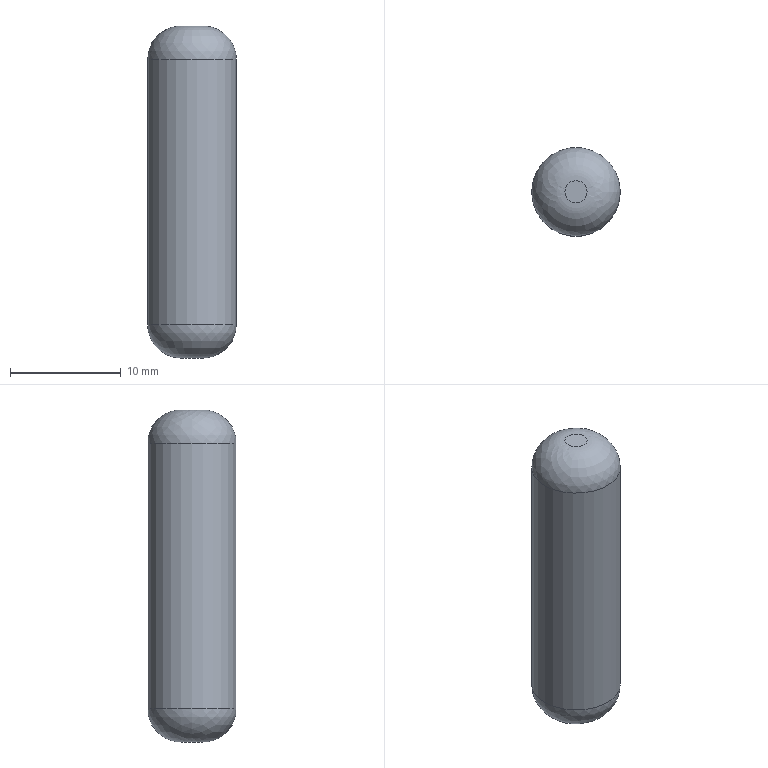Part | STEP file | 1 solid | 5 faces | box 8 x 8 x 30 mm | volume 1427 mm3 | plane 2 | spline 2 | cylinder 1 | commonest cylinder face diameters 8 x1
STEP:
#1=CARTESIAN_POINT('',(0.,0.,0.));
#2=DIRECTION('',(0.,0.,1.));
#3=DIRECTION('',(1.,0.,0.));
#4=AXIS2_PLACEMENT_3D('',#1,#2,#3);
#5=CARTESIAN_POINT('',(1518.247,357.48,-22.381));
#6=VERTEX_POINT('',#5);
#7=CARTESIAN_POINT('',(1517.247,357.48,-22.381));
#8=DIRECTION('',(0.,0.,1.));
#9=DIRECTION('',(1.,0.,0.));
#10=AXIS2_PLACEMENT_3D('',#7,#8,#9);
#11=CIRCLE('',#10,1.);
#12=CARTESIAN_POINT('',(1517.247,357.48,-22.381));
#13=DIRECTION('',(0.,0.,1.));
#14=DIRECTION('',(-1.,0.,0.));
#15=AXIS2_PLACEMENT_3D('',#12,#13,#14);
#16=PLANE('',#15);
#17=CARTESIAN_POINT('',(0.,0.));
#18=DIRECTION('',(-1.,0.));
#19=AXIS2_PLACEMENT_2D('',#17,#18);
#20=CIRCLE('',#19,1.);
#21=(GEOMETRIC_REPRESENTATION_CONTEXT(2)PARAMETRIC_REPRESENTATION_CONTEXT()REPRESENTATION_CONTEXT('',''));
#22=DEFINITIONAL_REPRESENTATION('',(#20),#21);
#23=PCURVE('',#16,#22);
#24=CARTESIAN_POINT('',(1518.247,357.48,-22.381));
#25=CARTESIAN_POINT('',(1518.247,359.48,-22.381));
#26=CARTESIAN_POINT('',(1516.247,359.48,-22.381));
#27=CARTESIAN_POINT('',(1516.247,357.48,-22.381));
#28=CARTESIAN_POINT('',(1516.247,355.48,-22.381));
#29=CARTESIAN_POINT('',(1518.247,355.48,-22.381));
#30=CARTESIAN_POINT('',(1518.247,357.48,-22.381));
#31=CARTESIAN_POINT('',(1520.005,357.48,-22.381));
#32=CARTESIAN_POINT('',(1520.005,362.995,-22.381));
#33=CARTESIAN_POINT('',(1514.49,362.995,-22.381));
#34=CARTESIAN_POINT('',(1514.49,357.48,-22.381));
#35=CARTESIAN_POINT('',(1514.49,351.966,-22.381));
#36=CARTESIAN_POINT('',(1520.005,351.966,-22.381));
#37=CARTESIAN_POINT('',(1520.005,357.48,-22.381));
#38=CARTESIAN_POINT('',(1521.247,357.48,-23.624));
#39=CARTESIAN_POINT('',(1521.247,365.48,-23.624));
#40=CARTESIAN_POINT('',(1513.247,365.48,-23.624));
#41=CARTESIAN_POINT('',(1513.247,357.48,-23.624));
#42=CARTESIAN_POINT('',(1513.247,349.48,-23.624));
#43=CARTESIAN_POINT('',(1521.247,349.48,-23.624));
#44=CARTESIAN_POINT('',(1521.247,357.48,-23.624));
#45=CARTESIAN_POINT('',(1521.247,357.48,-25.381));
#46=CARTESIAN_POINT('',(1521.247,365.48,-25.381));
#47=CARTESIAN_POINT('',(1513.247,365.48,-25.381));
#48=CARTESIAN_POINT('',(1513.247,357.48,-25.381));
#49=CARTESIAN_POINT('',(1513.247,349.48,-25.381));
#50=CARTESIAN_POINT('',(1521.247,349.48,-25.381));
#51=CARTESIAN_POINT('',(1521.247,357.48,-25.381));
#52=(BOUNDED_SURFACE()B_SPLINE_SURFACE(3,3,((#24,#25,#26,#27,#28,#29,#30),(#31,#32,#33,#34,#35,#36,#37),(#38,#39,#40,#41,#42,#43,#44),(#45,#46,#47,#48,#49,#50,#51)),.UNSPECIFIED.,.F.,.T.,.F.)B_SPLINE_SURFACE_WITH_KNOTS((4,4),(1,3,3,3,1),(0.,1.),(-0.5,0.,0.5,1.,1.5),.UNSPECIFIED.)GEOMETRIC_REPRESENTATION_ITEM()RATIONAL_B_SPLINE_SURFACE(((1.,0.3333,0.3333,1.,0.3333,0.3333,1.),(0.8047,0.2682,0.2682,0.8047,0.2682,0.2682,0.8047),(0.8047,0.2682,0.2682,0.8047,0.2682,0.2682,0.8047),(1.,0.3333,0.3333,1.,0.3333,0.3333,1.)))REPRESENTATION_ITEM('')SURFACE());
#53=CARTESIAN_POINT('',(0.,0.));
#54=CARTESIAN_POINT('',(0.,0.02352));
#55=CARTESIAN_POINT('',(0.,0.06491));
#56=CARTESIAN_POINT('',(0.,0.1146));
#57=CARTESIAN_POINT('',(0.,0.1575));
#58=CARTESIAN_POINT('',(0.,0.196));
#59=CARTESIAN_POINT('',(0.,0.2322));
#60=CARTESIAN_POINT('',(0.,0.2678));
#61=CARTESIAN_POINT('',(0.,0.304));
#62=CARTESIAN_POINT('',(0.,0.3425));
#63=CARTESIAN_POINT('',(0.,0.3856));
#64=CARTESIAN_POINT('',(0.,0.4343));
#65=CARTESIAN_POINT('',(0.,0.5));
#66=CARTESIAN_POINT('',(0.,0.5657));
#67=CARTESIAN_POINT('',(0.,0.6144));
#68=CARTESIAN_POINT('',(0.,0.6575));
#69=CARTESIAN_POINT('',(0.,0.696));
#70=CARTESIAN_POINT('',(0.,0.7322));
#71=CARTESIAN_POINT('',(0.,0.7678));
#72=CARTESIAN_POINT('',(0.,0.804));
#73=CARTESIAN_POINT('',(0.,0.8425));
#74=CARTESIAN_POINT('',(0.,0.8854));
#75=CARTESIAN_POINT('',(0.,0.9351));
#76=CARTESIAN_POINT('',(0.,0.9765));
#77=CARTESIAN_POINT('',(0.,1.));
#78=B_SPLINE_CURVE_WITH_KNOTS('',3,(#53,#54,#55,#56,#57,#58,#59,#60,#61,#62,#63,#64,#65,#66,#67,#68,#69,#70,#71,#72,#73,#74,#75,#76,#77),.UNSPECIFIED.,.F.,.F.,(4,1,1,1,1,1,1,1,1,1,1,1,1,1,1,1,1,1,1,1,1,1,4),(0.,0.2856,0.5712,0.8568,1.142,1.428,1.714,1.999,2.285,2.57,2.856,3.142,3.427,3.713,3.998,4.284,4.57,4.855,5.141,5.426,5.712,5.998,6.283),.QUASI_UNIFORM_KNOTS.);
#79=(GEOMETRIC_REPRESENTATION_CONTEXT(2)PARAMETRIC_REPRESENTATION_CONTEXT()REPRESENTATION_CONTEXT('',''));
#80=DEFINITIONAL_REPRESENTATION('',(#78),#79);
#81=PCURVE('',#52,#80);
#82=SURFACE_CURVE('',#11,(#23,#81),.PCURVE_S1.);
#83=EDGE_CURVE('',#6,#6,#82,.T.);
#84=ORIENTED_EDGE('',*,*,#83,.T.);
#85=EDGE_LOOP('',(#84));
#86=FACE_BOUND('',#85,.T.);
#87=ADVANCED_FACE('',(#86),#16,.T.);
#88=CARTESIAN_POINT('',(1516.247,357.48,-52.381));
#89=VERTEX_POINT('',#88);
#90=CARTESIAN_POINT('',(1517.247,357.48,-52.381));
#91=DIRECTION('',(0.,0.,-1.));
#92=DIRECTION('',(-1.,0.,0.));
#93=AXIS2_PLACEMENT_3D('',#90,#91,#92);
#94=CIRCLE('',#93,1.);
#95=CARTESIAN_POINT('',(1517.247,357.48,-52.381));
#96=DIRECTION('',(0.,0.,-1.));
#97=DIRECTION('',(1.,0.,0.));
#98=AXIS2_PLACEMENT_3D('',#95,#96,#97);
#99=PLANE('',#98);
#100=CARTESIAN_POINT('',(0.,0.));
#101=DIRECTION('',(-1.,0.));
#102=AXIS2_PLACEMENT_2D('',#100,#101);
#103=CIRCLE('',#102,1.);
#104=(GEOMETRIC_REPRESENTATION_CONTEXT(2)PARAMETRIC_REPRESENTATION_CONTEXT()REPRESENTATION_CONTEXT('',''));
#105=DEFINITIONAL_REPRESENTATION('',(#103),#104);
#106=PCURVE('',#99,#105);
#107=CARTESIAN_POINT('',(1516.247,357.48,-52.381));
#108=CARTESIAN_POINT('',(1516.247,359.48,-52.381));
#109=CARTESIAN_POINT('',(1518.247,359.48,-52.381));
#110=CARTESIAN_POINT('',(1518.247,357.48,-52.381));
#111=CARTESIAN_POINT('',(1518.247,355.48,-52.381));
#112=CARTESIAN_POINT('',(1516.247,355.48,-52.381));
#113=CARTESIAN_POINT('',(1516.247,357.48,-52.381));
#114=CARTESIAN_POINT('',(1514.49,357.48,-52.381));
#115=CARTESIAN_POINT('',(1514.49,362.995,-52.381));
#116=CARTESIAN_POINT('',(1520.005,362.995,-52.381));
#117=CARTESIAN_POINT('',(1520.005,357.48,-52.381));
#118=CARTESIAN_POINT('',(1520.005,351.966,-52.381));
#119=CARTESIAN_POINT('',(1514.49,351.966,-52.381));
#120=CARTESIAN_POINT('',(1514.49,357.48,-52.381));
#121=CARTESIAN_POINT('',(1513.247,357.48,-51.138));
#122=CARTESIAN_POINT('',(1513.247,365.48,-51.138));
#123=CARTESIAN_POINT('',(1521.247,365.48,-51.138));
#124=CARTESIAN_POINT('',(1521.247,357.48,-51.138));
#125=CARTESIAN_POINT('',(1521.247,349.48,-51.138));
#126=CARTESIAN_POINT('',(1513.247,349.48,-51.138));
#127=CARTESIAN_POINT('',(1513.247,357.48,-51.138));
#128=CARTESIAN_POINT('',(1513.247,357.48,-49.381));
#129=CARTESIAN_POINT('',(1513.247,365.48,-49.381));
#130=CARTESIAN_POINT('',(1521.247,365.48,-49.381));
#131=CARTESIAN_POINT('',(1521.247,357.48,-49.381));
#132=CARTESIAN_POINT('',(1521.247,349.48,-49.381));
#133=CARTESIAN_POINT('',(1513.247,349.48,-49.381));
#134=CARTESIAN_POINT('',(1513.247,357.48,-49.381));
#135=(BOUNDED_SURFACE()B_SPLINE_SURFACE(3,3,((#107,#108,#109,#110,#111,#112,#113),(#114,#115,#116,#117,#118,#119,#120),(#121,#122,#123,#124,#125,#126,#127),(#128,#129,#130,#131,#132,#133,#134)),.UNSPECIFIED.,.F.,.T.,.F.)B_SPLINE_SURFACE_WITH_KNOTS((4,4),(1,3,3,3,1),(0.,1.),(-0.5,0.,0.5,1.,1.5),.UNSPECIFIED.)GEOMETRIC_REPRESENTATION_ITEM()RATIONAL_B_SPLINE_SURFACE(((1.,0.3333,0.3333,1.,0.3333,0.3333,1.),(0.8047,0.2682,0.2682,0.8047,0.2682,0.2682,0.8047),(0.8047,0.2682,0.2682,0.8047,0.2682,0.2682,0.8047),(1.,0.3333,0.3333,1.,0.3333,0.3333,1.)))REPRESENTATION_ITEM('')SURFACE());
#136=CARTESIAN_POINT('',(0.,0.));
#137=CARTESIAN_POINT('',(0.,0.02352));
#138=CARTESIAN_POINT('',(0.,0.06491));
#139=CARTESIAN_POINT('',(0.,0.1146));
#140=CARTESIAN_POINT('',(0.,0.1575));
#141=CARTESIAN_POINT('',(0.,0.196));
#142=CARTESIAN_POINT('',(0.,0.2322));
#143=CARTESIAN_POINT('',(0.,0.2678));
#144=CARTESIAN_POINT('',(0.,0.304));
#145=CARTESIAN_POINT('',(0.,0.3425));
#146=CARTESIAN_POINT('',(0.,0.3856));
#147=CARTESIAN_POINT('',(0.,0.4343));
#148=CARTESIAN_POINT('',(0.,0.5));
#149=CARTESIAN_POINT('',(0.,0.5657));
#150=CARTESIAN_POINT('',(0.,0.6144));
#151=CARTESIAN_POINT('',(0.,0.6575));
#152=CARTESIAN_POINT('',(0.,0.696));
#153=CARTESIAN_POINT('',(0.,0.7322));
#154=CARTESIAN_POINT('',(0.,0.7678));
#155=CARTESIAN_POINT('',(0.,0.804));
#156=CARTESIAN_POINT('',(0.,0.8425));
#157=CARTESIAN_POINT('',(0.,0.8854));
#158=CARTESIAN_POINT('',(0.,0.9351));
#159=CARTESIAN_POINT('',(0.,0.9765));
#160=CARTESIAN_POINT('',(0.,1.));
#161=B_SPLINE_CURVE_WITH_KNOTS('',3,(#136,#137,#138,#139,#140,#141,#142,#143,#144,#145,#146,#147,#148,#149,#150,#151,#152,#153,#154,#155,#156,#157,#158,#159,#160),.UNSPECIFIED.,.F.,.F.,(4,1,1,1,1,1,1,1,1,1,1,1,1,1,1,1,1,1,1,1,1,1,4),(0.,0.2856,0.5712,0.8568,1.142,1.428,1.714,1.999,2.285,2.57,2.856,3.142,3.427,3.713,3.998,4.284,4.57,4.855,5.141,5.426,5.712,5.998,6.283),.QUASI_UNIFORM_KNOTS.);
#162=(GEOMETRIC_REPRESENTATION_CONTEXT(2)PARAMETRIC_REPRESENTATION_CONTEXT()REPRESENTATION_CONTEXT('',''));
#163=DEFINITIONAL_REPRESENTATION('',(#161),#162);
#164=PCURVE('',#135,#163);
#165=SURFACE_CURVE('',#94,(#106,#164),.PCURVE_S1.);
#166=EDGE_CURVE('',#89,#89,#165,.T.);
#167=ORIENTED_EDGE('',*,*,#166,.T.);
#168=EDGE_LOOP('',(#167));
#169=FACE_BOUND('',#168,.T.);
#170=ADVANCED_FACE('',(#169),#99,.T.);
#171=CARTESIAN_POINT('',(1513.247,357.48,-49.381));
#172=VERTEX_POINT('',#171);
#173=CARTESIAN_POINT('',(1517.247,357.48,-49.381));
#174=DIRECTION('',(0.,0.,1.));
#175=DIRECTION('',(-1.,0.,0.));
#176=AXIS2_PLACEMENT_3D('',#173,#174,#175);
#177=CIRCLE('',#176,4.);
#178=CARTESIAN_POINT('',(1517.247,357.48,-47.381));
#179=DIRECTION('',(0.,0.,1.));
#180=DIRECTION('',(-1.,0.,0.));
#181=AXIS2_PLACEMENT_3D('',#178,#179,#180);
#182=CYLINDRICAL_SURFACE('',#181,4.);
#183=CARTESIAN_POINT('',(0.,-2.));
#184=DIRECTION('',(1.,0.));
#185=VECTOR('',#184,1.);
#186=LINE('',#183,#185);
#187=(GEOMETRIC_REPRESENTATION_CONTEXT(2)PARAMETRIC_REPRESENTATION_CONTEXT()REPRESENTATION_CONTEXT('',''));
#188=DEFINITIONAL_REPRESENTATION('',(#186),#187);
#189=PCURVE('',#182,#188);
#190=CARTESIAN_POINT('',(1.,1.));
#191=CARTESIAN_POINT('',(1.,0.9765));
#192=CARTESIAN_POINT('',(1.,0.9351));
#193=CARTESIAN_POINT('',(1.,0.8854));
#194=CARTESIAN_POINT('',(1.,0.8425));
#195=CARTESIAN_POINT('',(1.,0.804));
#196=CARTESIAN_POINT('',(1.,0.7678));
#197=CARTESIAN_POINT('',(1.,0.7322));
#198=CARTESIAN_POINT('',(1.,0.696));
#199=CARTESIAN_POINT('',(1.,0.6575));
#200=CARTESIAN_POINT('',(1.,0.6144));
#201=CARTESIAN_POINT('',(1.,0.5657));
#202=CARTESIAN_POINT('',(1.,0.5));
#203=CARTESIAN_POINT('',(1.,0.4343));
#204=CARTESIAN_POINT('',(1.,0.3856));
#205=CARTESIAN_POINT('',(1.,0.3425));
#206=CARTESIAN_POINT('',(1.,0.304));
#207=CARTESIAN_POINT('',(1.,0.2678));
#208=CARTESIAN_POINT('',(1.,0.2322));
#209=CARTESIAN_POINT('',(1.,0.196));
#210=CARTESIAN_POINT('',(1.,0.1575));
#211=CARTESIAN_POINT('',(1.,0.1146));
#212=CARTESIAN_POINT('',(1.,0.06491));
#213=CARTESIAN_POINT('',(1.,0.02352));
#214=CARTESIAN_POINT('',(1.,0.));
#215=B_SPLINE_CURVE_WITH_KNOTS('',3,(#190,#191,#192,#193,#194,#195,#196,#197,#198,#199,#200,#201,#202,#203,#204,#205,#206,#207,#208,#209,#210,#211,#212,#213,#214),.UNSPECIFIED.,.F.,.F.,(4,1,1,1,1,1,1,1,1,1,1,1,1,1,1,1,1,1,1,1,1,1,4),(0.,0.2856,0.5712,0.8568,1.142,1.428,1.714,1.999,2.285,2.57,2.856,3.142,3.427,3.713,3.998,4.284,4.57,4.855,5.141,5.426,5.712,5.998,6.283),.QUASI_UNIFORM_KNOTS.);
#216=(GEOMETRIC_REPRESENTATION_CONTEXT(2)PARAMETRIC_REPRESENTATION_CONTEXT()REPRESENTATION_CONTEXT('',''));
#217=DEFINITIONAL_REPRESENTATION('',(#215),#216);
#218=PCURVE('',#135,#217);
#219=SURFACE_CURVE('',#177,(#189,#218),.PCURVE_S1.);
#220=EDGE_CURVE('',#172,#172,#219,.T.);
#221=ORIENTED_EDGE('',*,*,#220,.T.);
#222=CARTESIAN_POINT('',(1513.247,357.48,-25.381));
#223=VERTEX_POINT('',#222);
#224=CARTESIAN_POINT('',(1513.247,357.48,-49.381));
#225=CARTESIAN_POINT('',(1513.247,357.48,-25.381));
#226=B_SPLINE_CURVE_WITH_KNOTS('',1,(#224,#225),.UNSPECIFIED.,.F.,.F.,(2,2),(-2.,22.),.PIECEWISE_BEZIER_KNOTS.);
#227=CARTESIAN_POINT('',(6.283,0.));
#228=DIRECTION('',(0.,1.));
#229=VECTOR('',#228,1.);
#230=LINE('',#227,#229);
#231=(GEOMETRIC_REPRESENTATION_CONTEXT(2)PARAMETRIC_REPRESENTATION_CONTEXT()REPRESENTATION_CONTEXT('',''));
#232=DEFINITIONAL_REPRESENTATION('',(#230),#231);
#233=PCURVE('',#182,#232);
#234=CARTESIAN_POINT('',(0.,0.));
#235=DIRECTION('',(0.,1.));
#236=VECTOR('',#235,1.);
#237=LINE('',#234,#236);
#238=(GEOMETRIC_REPRESENTATION_CONTEXT(2)PARAMETRIC_REPRESENTATION_CONTEXT()REPRESENTATION_CONTEXT('',''));
#239=DEFINITIONAL_REPRESENTATION('',(#237),#238);
#240=PCURVE('',#182,#239);
#241=SEAM_CURVE('',#226,(#233,#240),.PCURVE_S1.);
#242=EDGE_CURVE('',#172,#223,#241,.T.);
#243=ORIENTED_EDGE('',*,*,#242,.T.);
#244=CARTESIAN_POINT('',(1521.247,357.48,-25.381));
#245=VERTEX_POINT('',#244);
#246=CARTESIAN_POINT('',(1517.247,357.48,-25.381));
#247=DIRECTION('',(0.,0.,-1.));
#248=DIRECTION('',(1.,0.,0.));
#249=AXIS2_PLACEMENT_3D('',#246,#247,#248);
#250=CIRCLE('',#249,4.);
#251=CARTESIAN_POINT('',(9.425,22.));
#252=DIRECTION('',(-1.,0.));
#253=VECTOR('',#252,1.);
#254=LINE('',#251,#253);
#255=(GEOMETRIC_REPRESENTATION_CONTEXT(2)PARAMETRIC_REPRESENTATION_CONTEXT()REPRESENTATION_CONTEXT('',''));
#256=DEFINITIONAL_REPRESENTATION('',(#254),#255);
#257=PCURVE('',#182,#256);
#258=CARTESIAN_POINT('',(1.,0.5));
#259=CARTESIAN_POINT('',(1.,0.4881));
#260=CARTESIAN_POINT('',(1.,0.466));
#261=CARTESIAN_POINT('',(1.,0.4367));
#262=CARTESIAN_POINT('',(1.,0.4103));
#263=CARTESIAN_POINT('',(1.,0.3862));
#264=CARTESIAN_POINT('',(1.,0.3639));
#265=CARTESIAN_POINT('',(1.,0.3431));
#266=CARTESIAN_POINT('',(1.,0.3233));
#267=CARTESIAN_POINT('',(1.,0.3043));
#268=CARTESIAN_POINT('',(1.,0.2859));
#269=CARTESIAN_POINT('',(1.,0.2678));
#270=CARTESIAN_POINT('',(1.,0.25));
#271=CARTESIAN_POINT('',(1.,0.2322));
#272=CARTESIAN_POINT('',(1.,0.2141));
#273=CARTESIAN_POINT('',(1.,0.1957));
#274=CARTESIAN_POINT('',(1.,0.1767));
#275=CARTESIAN_POINT('',(1.,0.1569));
#276=CARTESIAN_POINT('',(1.,0.1361));
#277=CARTESIAN_POINT('',(1.,0.1138));
#278=CARTESIAN_POINT('',(1.,0.08972));
#279=CARTESIAN_POINT('',(1.,0.06334));
#280=CARTESIAN_POINT('',(1.,0.03403));
#281=CARTESIAN_POINT('',(1.,0.01187));
#282=CARTESIAN_POINT('',(1.,0.));
#283=B_SPLINE_CURVE_WITH_KNOTS('',3,(#258,#259,#260,#261,#262,#263,#264,#265,#266,#267,#268,#269,#270,#271,#272,#273,#274,#275,#276,#277,#278,#279,#280,#281,#282),.UNSPECIFIED.,.F.,.F.,(4,1,1,1,1,1,1,1,1,1,1,1,1,1,1,1,1,1,1,1,1,1,4),(3.142,3.284,3.427,3.57,3.713,3.856,3.998,4.141,4.284,4.427,4.57,4.712,4.855,4.998,5.141,5.284,5.426,5.569,5.712,5.855,5.998,6.14,6.283),.QUASI_UNIFORM_KNOTS.);
#284=(GEOMETRIC_REPRESENTATION_CONTEXT(2)PARAMETRIC_REPRESENTATION_CONTEXT()REPRESENTATION_CONTEXT('',''));
#285=DEFINITIONAL_REPRESENTATION('',(#283),#284);
#286=PCURVE('',#52,#285);
#287=SURFACE_CURVE('',#250,(#257,#286),.PCURVE_S1.);
#288=EDGE_CURVE('',#223,#245,#287,.T.);
#289=ORIENTED_EDGE('',*,*,#288,.T.);
#290=CARTESIAN_POINT('',(1517.247,357.48,-25.381));
#291=DIRECTION('',(0.,0.,-1.));
#292=DIRECTION('',(1.,0.,0.));
#293=AXIS2_PLACEMENT_3D('',#290,#291,#292);
#294=CIRCLE('',#293,4.);
#295=CARTESIAN_POINT('',(3.142,22.));
#296=DIRECTION('',(-1.,0.));
#297=VECTOR('',#296,1.);
#298=LINE('',#295,#297);
#299=(GEOMETRIC_REPRESENTATION_CONTEXT(2)PARAMETRIC_REPRESENTATION_CONTEXT()REPRESENTATION_CONTEXT('',''));
#300=DEFINITIONAL_REPRESENTATION('',(#298),#299);
#301=PCURVE('',#182,#300);
#302=CARTESIAN_POINT('',(1.,1.));
#303=CARTESIAN_POINT('',(1.,0.9881));
#304=CARTESIAN_POINT('',(1.,0.966));
#305=CARTESIAN_POINT('',(1.,0.9367));
#306=CARTESIAN_POINT('',(1.,0.9103));
#307=CARTESIAN_POINT('',(1.,0.8862));
#308=CARTESIAN_POINT('',(1.,0.8639));
#309=CARTESIAN_POINT('',(1.,0.8431));
#310=CARTESIAN_POINT('',(1.,0.8233));
#311=CARTESIAN_POINT('',(1.,0.8043));
#312=CARTESIAN_POINT('',(1.,0.7859));
#313=CARTESIAN_POINT('',(1.,0.7678));
#314=CARTESIAN_POINT('',(1.,0.75));
#315=CARTESIAN_POINT('',(1.,0.7322));
#316=CARTESIAN_POINT('',(1.,0.7141));
#317=CARTESIAN_POINT('',(1.,0.6957));
#318=CARTESIAN_POINT('',(1.,0.6767));
#319=CARTESIAN_POINT('',(1.,0.6569));
#320=CARTESIAN_POINT('',(1.,0.6361));
#321=CARTESIAN_POINT('',(1.,0.6138));
#322=CARTESIAN_POINT('',(1.,0.5897));
#323=CARTESIAN_POINT('',(1.,0.5633));
#324=CARTESIAN_POINT('',(1.,0.534));
#325=CARTESIAN_POINT('',(1.,0.5119));
#326=CARTESIAN_POINT('',(1.,0.5));
#327=B_SPLINE_CURVE_WITH_KNOTS('',3,(#302,#303,#304,#305,#306,#307,#308,#309,#310,#311,#312,#313,#314,#315,#316,#317,#318,#319,#320,#321,#322,#323,#324,#325,#326),.UNSPECIFIED.,.F.,.F.,(4,1,1,1,1,1,1,1,1,1,1,1,1,1,1,1,1,1,1,1,1,1,4),(0.,0.1428,0.2856,0.4284,0.5712,0.714,0.8568,0.9996,1.142,1.285,1.428,1.571,1.714,1.856,1.999,2.142,2.285,2.428,2.57,2.713,2.856,2.999,3.142),.QUASI_UNIFORM_KNOTS.);
#328=(GEOMETRIC_REPRESENTATION_CONTEXT(2)PARAMETRIC_REPRESENTATION_CONTEXT()REPRESENTATION_CONTEXT('',''));
#329=DEFINITIONAL_REPRESENTATION('',(#327),#328);
#330=PCURVE('',#52,#329);
#331=SURFACE_CURVE('',#294,(#301,#330),.PCURVE_S1.);
#332=EDGE_CURVE('',#245,#223,#331,.T.);
#333=ORIENTED_EDGE('',*,*,#332,.T.);
#334=ORIENTED_EDGE('',*,*,#242,.F.);
#335=EDGE_LOOP('',(#221,#243,#289,#333,#334));
#336=FACE_BOUND('',#335,.T.);
#337=ADVANCED_FACE('',(#336),#182,.T.);
#338=ORIENTED_EDGE('',*,*,#166,.F.);
#339=CARTESIAN_POINT('',(1516.247,357.48,-52.381));
#340=CARTESIAN_POINT('',(1514.49,357.48,-52.381));
#341=CARTESIAN_POINT('',(1513.247,357.48,-51.138));
#342=CARTESIAN_POINT('',(1513.247,357.48,-49.381));
#343=(BOUNDED_CURVE()B_SPLINE_CURVE(3,(#339,#340,#341,#342),.UNSPECIFIED.,.F.,.F.)B_SPLINE_CURVE_WITH_KNOTS((4,4),(0.,1.),.PIECEWISE_BEZIER_KNOTS.)CURVE()GEOMETRIC_REPRESENTATION_ITEM()RATIONAL_B_SPLINE_CURVE((1.,0.8047,0.8047,1.))REPRESENTATION_ITEM(''));
#344=CARTESIAN_POINT('',(0.,0.));
#345=DIRECTION('',(1.,0.));
#346=VECTOR('',#345,1.);
#347=LINE('',#344,#346);
#348=(GEOMETRIC_REPRESENTATION_CONTEXT(2)PARAMETRIC_REPRESENTATION_CONTEXT()REPRESENTATION_CONTEXT('',''));
#349=DEFINITIONAL_REPRESENTATION('',(#347),#348);
#350=PCURVE('',#135,#349);
#351=CARTESIAN_POINT('',(0.,1.));
#352=DIRECTION('',(1.,0.));
#353=VECTOR('',#352,1.);
#354=LINE('',#351,#353);
#355=(GEOMETRIC_REPRESENTATION_CONTEXT(2)PARAMETRIC_REPRESENTATION_CONTEXT()REPRESENTATION_CONTEXT('',''));
#356=DEFINITIONAL_REPRESENTATION('',(#354),#355);
#357=PCURVE('',#135,#356);
#358=SEAM_CURVE('',#343,(#350,#357),.PCURVE_S1.);
#359=EDGE_CURVE('',#89,#172,#358,.T.);
#360=ORIENTED_EDGE('',*,*,#359,.T.);
#361=ORIENTED_EDGE('',*,*,#220,.F.);
#362=ORIENTED_EDGE('',*,*,#359,.F.);
#363=EDGE_LOOP('',(#338,#360,#361,#362));
#364=FACE_BOUND('',#363,.T.);
#365=ADVANCED_FACE('',(#364),#135,.T.);
#366=ORIENTED_EDGE('',*,*,#83,.F.);
#367=CARTESIAN_POINT('',(1518.247,357.48,-22.381));
#368=CARTESIAN_POINT('',(1520.005,357.48,-22.381));
#369=CARTESIAN_POINT('',(1521.247,357.48,-23.624));
#370=CARTESIAN_POINT('',(1521.247,357.48,-25.381));
#371=(BOUNDED_CURVE()B_SPLINE_CURVE(3,(#367,#368,#369,#370),.UNSPECIFIED.,.F.,.F.)B_SPLINE_CURVE_WITH_KNOTS((4,4),(0.,1.),.PIECEWISE_BEZIER_KNOTS.)CURVE()GEOMETRIC_REPRESENTATION_ITEM()RATIONAL_B_SPLINE_CURVE((1.,0.8047,0.8047,1.))REPRESENTATION_ITEM(''));
#372=CARTESIAN_POINT('',(0.,0.));
#373=DIRECTION('',(1.,0.));
#374=VECTOR('',#373,1.);
#375=LINE('',#372,#374);
#376=(GEOMETRIC_REPRESENTATION_CONTEXT(2)PARAMETRIC_REPRESENTATION_CONTEXT()REPRESENTATION_CONTEXT('',''));
#377=DEFINITIONAL_REPRESENTATION('',(#375),#376);
#378=PCURVE('',#52,#377);
#379=CARTESIAN_POINT('',(0.,1.));
#380=DIRECTION('',(1.,0.));
#381=VECTOR('',#380,1.);
#382=LINE('',#379,#381);
#383=(GEOMETRIC_REPRESENTATION_CONTEXT(2)PARAMETRIC_REPRESENTATION_CONTEXT()REPRESENTATION_CONTEXT('',''));
#384=DEFINITIONAL_REPRESENTATION('',(#382),#383);
#385=PCURVE('',#52,#384);
#386=SEAM_CURVE('',#371,(#378,#385),.PCURVE_S1.);
#387=EDGE_CURVE('',#6,#245,#386,.T.);
#388=ORIENTED_EDGE('',*,*,#387,.T.);
#389=ORIENTED_EDGE('',*,*,#288,.F.);
#390=ORIENTED_EDGE('',*,*,#332,.F.);
#391=ORIENTED_EDGE('',*,*,#387,.F.);
#392=EDGE_LOOP('',(#366,#388,#389,#390,#391));
#393=FACE_BOUND('',#392,.T.);
#394=ADVANCED_FACE('',(#393),#52,.T.);
#395=CLOSED_SHELL('',(#87,#170,#337,#365,#394));
#396=MANIFOLD_SOLID_BREP('',#395);
#397=(LENGTH_UNIT()NAMED_UNIT(*)SI_UNIT(.MILLI.,.METRE.));
#398=UNCERTAINTY_MEASURE_WITH_UNIT(LENGTH_MEASURE(0.00001),#397,'','');
#399=(NAMED_UNIT(*)PLANE_ANGLE_UNIT()SI_UNIT($,.RADIAN.));
#400=(NAMED_UNIT(*)SI_UNIT($,.STERADIAN.)SOLID_ANGLE_UNIT());
#401=(GEOMETRIC_REPRESENTATION_CONTEXT(3)GLOBAL_UNCERTAINTY_ASSIGNED_CONTEXT((#398))GLOBAL_UNIT_ASSIGNED_CONTEXT((#397,#399,#400))REPRESENTATION_CONTEXT('',''));
#402=ADVANCED_BREP_SHAPE_REPRESENTATION('',(#4,#396),#401);